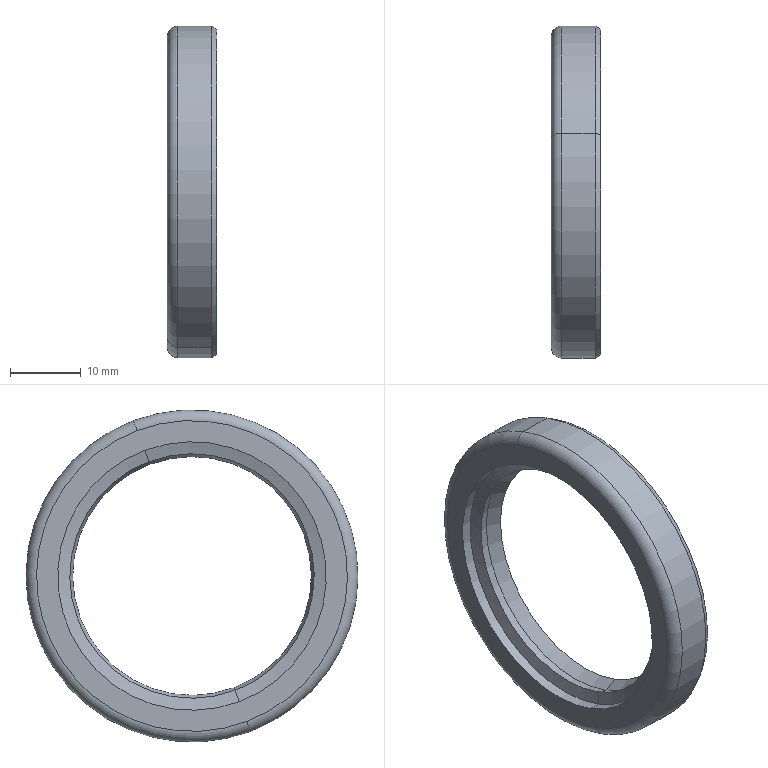Part | SolidWorks | features BaseBody 1 | 1 solid | 34 faces | box 7 x 47 x 47 mm | volume 3647 mm3 | cone 10 | cylinder 10 | torus 8 | plane 6 | commonest cylinder face diameters 38 x2 40 x2 41.6 x2 44 x2 47 x2
STEP:
#1=CARTESIAN_POINT('',(-6.4,6.861,18.253));
#2=VERTEX_POINT('',#1);
#3=CARTESIAN_POINT('',(-7.3,6.544,17.411));
#4=VERTEX_POINT('',#3);
#5=CARTESIAN_POINT('',(-7.3,6.861,18.253));
#6=DIRECTION('',(0.,0.9361,-0.3518));
#7=DIRECTION('',(0.,0.3518,0.9361));
#8=AXIS2_PLACEMENT_3D('',#5,#6,#7);
#9=CIRCLE('',#8,0.9);
#10=EDGE_CURVE('',#2,#4,#9,.T.);
#11=ORIENTED_EDGE('',*,*,#10,.T.);
#12=CARTESIAN_POINT('',(-7.3,-6.544,-17.411));
#13=VERTEX_POINT('',#12);
#14=CARTESIAN_POINT('',(-7.3,0.,0.));
#15=DIRECTION('',(1.,0.,0.));
#16=DIRECTION('',(0.,0.,-1.));
#17=AXIS2_PLACEMENT_3D('',#14,#15,#16);
#18=CIRCLE('',#17,18.6);
#19=EDGE_CURVE('',#4,#13,#18,.T.);
#20=ORIENTED_EDGE('',*,*,#19,.T.);
#21=CARTESIAN_POINT('',(-6.4,-6.861,-18.253));
#22=VERTEX_POINT('',#21);
#23=CARTESIAN_POINT('',(-7.3,-6.861,-18.253));
#24=DIRECTION('',(0.,-0.9361,0.3518));
#25=DIRECTION('',(0.,-0.3518,-0.9361));
#26=AXIS2_PLACEMENT_3D('',#23,#24,#25);
#27=CIRCLE('',#26,0.9);
#28=EDGE_CURVE('',#22,#13,#27,.T.);
#29=ORIENTED_EDGE('',*,*,#28,.F.);
#30=CARTESIAN_POINT('',(-6.4,0.,0.));
#31=DIRECTION('',(1.,0.,0.));
#32=DIRECTION('',(0.,0.3518,0.9361));
#33=AXIS2_PLACEMENT_3D('',#30,#31,#32);
#34=CIRCLE('',#33,19.5);
#35=EDGE_CURVE('',#2,#22,#34,.T.);
#36=ORIENTED_EDGE('',*,*,#35,.F.);
#37=EDGE_LOOP('',(#11,#20,#29,#36));
#38=FACE_OUTER_BOUND('',#37,.T.);
#39=CARTESIAN_POINT('',(-7.3,0.,0.));
#40=DIRECTION('',(1.,0.,0.));
#41=DIRECTION('',(0.,0.3518,0.9361));
#42=AXIS2_PLACEMENT_3D('',#39,#40,#41);
#43=TOROIDAL_SURFACE('',#42,19.5,0.9);
#44=ADVANCED_FACE('',(#38),#43,.F.);
#45=ORIENTED_EDGE('',*,*,#28,.T.);
#46=CARTESIAN_POINT('',(-7.3,0.,0.));
#47=DIRECTION('',(1.,0.,0.));
#48=DIRECTION('',(0.,0.,-1.));
#49=AXIS2_PLACEMENT_3D('',#46,#47,#48);
#50=CIRCLE('',#49,18.6);
#51=EDGE_CURVE('',#13,#4,#50,.T.);
#52=ORIENTED_EDGE('',*,*,#51,.T.);
#53=ORIENTED_EDGE('',*,*,#10,.F.);
#54=CARTESIAN_POINT('',(-6.4,0.,0.));
#55=DIRECTION('',(1.,0.,0.));
#56=DIRECTION('',(0.,0.3518,0.9361));
#57=AXIS2_PLACEMENT_3D('',#54,#55,#56);
#58=CIRCLE('',#57,19.5);
#59=EDGE_CURVE('',#22,#2,#58,.T.);
#60=ORIENTED_EDGE('',*,*,#59,.F.);
#61=EDGE_LOOP('',(#45,#52,#53,#60));
#62=FACE_OUTER_BOUND('',#61,.T.);
#63=CARTESIAN_POINT('',(-7.3,0.,0.));
#64=DIRECTION('',(1.,0.,0.));
#65=DIRECTION('',(0.,0.3518,0.9361));
#66=AXIS2_PLACEMENT_3D('',#63,#64,#65);
#67=TOROIDAL_SURFACE('',#66,19.5,0.9);
#68=ADVANCED_FACE('',(#62),#67,.F.);
#69=CARTESIAN_POINT('',(-12.,-7.741,-20.593));
#70=VERTEX_POINT('',#69);
#71=CARTESIAN_POINT('',(-12.,7.741,20.593));
#72=VERTEX_POINT('',#71);
#73=CARTESIAN_POINT('',(-12.,0.,0.));
#74=DIRECTION('',(-1.,0.,0.));
#75=DIRECTION('',(0.,0.3518,0.9361));
#76=AXIS2_PLACEMENT_3D('',#73,#74,#75);
#77=CIRCLE('',#76,22.);
#78=EDGE_CURVE('',#70,#72,#77,.T.);
#79=ORIENTED_EDGE('',*,*,#78,.F.);
#80=CARTESIAN_POINT('',(-10.5,-8.268,-21.997));
#81=VERTEX_POINT('',#80);
#82=CARTESIAN_POINT('',(-10.5,-7.741,-20.593));
#83=DIRECTION('',(0.,-0.9361,0.3518));
#84=DIRECTION('',(0.,-0.3518,-0.9361));
#85=AXIS2_PLACEMENT_3D('',#82,#83,#84);
#86=CIRCLE('',#85,1.5);
#87=EDGE_CURVE('',#70,#81,#86,.T.);
#88=ORIENTED_EDGE('',*,*,#87,.T.);
#89=CARTESIAN_POINT('',(-10.5,8.268,21.997));
#90=VERTEX_POINT('',#89);
#91=CARTESIAN_POINT('',(-10.5,0.,0.));
#92=DIRECTION('',(1.,0.,0.));
#93=DIRECTION('',(0.,0.3518,0.9361));
#94=AXIS2_PLACEMENT_3D('',#91,#92,#93);
#95=CIRCLE('',#94,23.5);
#96=EDGE_CURVE('',#90,#81,#95,.T.);
#97=ORIENTED_EDGE('',*,*,#96,.F.);
#98=CARTESIAN_POINT('',(-10.5,7.741,20.593));
#99=DIRECTION('',(0.,0.9361,-0.3518));
#100=DIRECTION('',(0.,0.3518,0.9361));
#101=AXIS2_PLACEMENT_3D('',#98,#99,#100);
#102=CIRCLE('',#101,1.5);
#103=EDGE_CURVE('',#72,#90,#102,.T.);
#104=ORIENTED_EDGE('',*,*,#103,.F.);
#105=EDGE_LOOP('',(#79,#88,#97,#104));
#106=FACE_OUTER_BOUND('',#105,.T.);
#107=CARTESIAN_POINT('',(-10.5,0.,0.));
#108=DIRECTION('',(1.,0.,0.));
#109=DIRECTION('',(0.,0.3518,0.9361));
#110=AXIS2_PLACEMENT_3D('',#107,#108,#109);
#111=TOROIDAL_SURFACE('',#110,22.,1.5);
#112=ADVANCED_FACE('',(#106),#111,.T.);
#113=CARTESIAN_POINT('',(-8.7,7.741,20.593));
#114=VERTEX_POINT('',#113);
#115=CARTESIAN_POINT('',(-8.7,-7.741,-20.593));
#116=VERTEX_POINT('',#115);
#117=CARTESIAN_POINT('',(-8.7,0.,0.));
#118=DIRECTION('',(-1.,0.,0.));
#119=DIRECTION('',(0.,-0.3518,-0.9361));
#120=AXIS2_PLACEMENT_3D('',#117,#118,#119);
#121=CIRCLE('',#120,22.);
#122=EDGE_CURVE('',#114,#116,#121,.T.);
#123=ORIENTED_EDGE('',*,*,#122,.F.);
#124=CARTESIAN_POINT('',(-9.,7.635,20.312));
#125=VERTEX_POINT('',#124);
#126=CARTESIAN_POINT('',(-8.7,7.635,20.312));
#127=DIRECTION('',(0.,-0.9361,0.3518));
#128=DIRECTION('',(0.,-0.3518,-0.9361));
#129=AXIS2_PLACEMENT_3D('',#126,#127,#128);
#130=CIRCLE('',#129,0.3);
#131=EDGE_CURVE('',#114,#125,#130,.T.);
#132=ORIENTED_EDGE('',*,*,#131,.T.);
#133=CARTESIAN_POINT('',(-9.,-7.635,-20.312));
#134=VERTEX_POINT('',#133);
#135=CARTESIAN_POINT('',(-9.,0.,0.));
#136=DIRECTION('',(1.,0.,0.));
#137=DIRECTION('',(0.,-0.3518,-0.9361));
#138=AXIS2_PLACEMENT_3D('',#135,#136,#137);
#139=CIRCLE('',#138,21.7);
#140=EDGE_CURVE('',#134,#125,#139,.T.);
#141=ORIENTED_EDGE('',*,*,#140,.F.);
#142=CARTESIAN_POINT('',(-8.7,-7.635,-20.312));
#143=DIRECTION('',(0.,0.9361,-0.3518));
#144=DIRECTION('',(0.,0.3518,0.9361));
#145=AXIS2_PLACEMENT_3D('',#142,#143,#144);
#146=CIRCLE('',#145,0.3);
#147=EDGE_CURVE('',#116,#134,#146,.T.);
#148=ORIENTED_EDGE('',*,*,#147,.F.);
#149=EDGE_LOOP('',(#123,#132,#141,#148));
#150=FACE_OUTER_BOUND('',#149,.T.);
#151=CARTESIAN_POINT('',(-8.7,0.,0.));
#152=DIRECTION('',(-1.,0.,0.));
#153=DIRECTION('',(0.,-0.3518,-0.9361));
#154=AXIS2_PLACEMENT_3D('',#151,#152,#153);
#155=TOROIDAL_SURFACE('',#154,21.7,0.3);
#156=ADVANCED_FACE('',(#150),#155,.F.);
#157=CARTESIAN_POINT('',(-5.,8.106,21.565));
#158=VERTEX_POINT('',#157);
#159=CARTESIAN_POINT('',(-5.,-8.106,-21.565));
#160=VERTEX_POINT('',#159);
#161=CARTESIAN_POINT('',(-5.,0.,0.));
#162=DIRECTION('',(1.,0.,0.));
#163=DIRECTION('',(0.,-0.3518,-0.9361));
#164=AXIS2_PLACEMENT_3D('',#161,#162,#163);
#165=CIRCLE('',#164,23.038);
#166=EDGE_CURVE('',#158,#160,#165,.T.);
#167=ORIENTED_EDGE('',*,*,#166,.F.);
#168=CARTESIAN_POINT('',(-5.8,8.268,21.997));
#169=VERTEX_POINT('',#168);
#170=CARTESIAN_POINT('',(-5.,8.106,21.565));
#171=DIRECTION('',(-0.866,0.1759,0.468));
#172=VECTOR('',#171,1000.);
#173=LINE('',#170,#172);
#174=EDGE_CURVE('',#158,#169,#173,.T.);
#175=ORIENTED_EDGE('',*,*,#174,.T.);
#176=CARTESIAN_POINT('',(-5.8,-8.268,-21.997));
#177=VERTEX_POINT('',#176);
#178=CARTESIAN_POINT('',(-5.8,0.,0.));
#179=DIRECTION('',(-1.,0.,0.));
#180=DIRECTION('',(0.,-0.3518,-0.9361));
#181=AXIS2_PLACEMENT_3D('',#178,#179,#180);
#182=CIRCLE('',#181,23.5);
#183=EDGE_CURVE('',#177,#169,#182,.T.);
#184=ORIENTED_EDGE('',*,*,#183,.F.);
#185=CARTESIAN_POINT('',(-5.,-8.106,-21.565));
#186=DIRECTION('',(-0.866,-0.1759,-0.468));
#187=VECTOR('',#186,1000.);
#188=LINE('',#185,#187);
#189=EDGE_CURVE('',#160,#177,#188,.T.);
#190=ORIENTED_EDGE('',*,*,#189,.F.);
#191=EDGE_LOOP('',(#167,#175,#184,#190));
#192=FACE_OUTER_BOUND('',#191,.T.);
#193=CARTESIAN_POINT('',(-5.,0.,0.));
#194=DIRECTION('',(-1.,0.,0.));
#195=DIRECTION('',(0.,-0.3518,-0.9361));
#196=AXIS2_PLACEMENT_3D('',#193,#194,#195);
#197=CONICAL_SURFACE('',#196,23.038,0.5236);
#198=ADVANCED_FACE('',(#192),#197,.T.);
#199=CARTESIAN_POINT('',(-9.,7.318,19.47));
#200=VERTEX_POINT('',#199);
#201=CARTESIAN_POINT('',(-9.,-7.318,-19.47));
#202=VERTEX_POINT('',#201);
#203=CARTESIAN_POINT('',(-9.,0.,0.));
#204=DIRECTION('',(1.,0.,0.));
#205=DIRECTION('',(0.,0.3518,0.9361));
#206=AXIS2_PLACEMENT_3D('',#203,#204,#205);
#207=CIRCLE('',#206,20.8);
#208=EDGE_CURVE('',#200,#202,#207,.T.);
#209=ORIENTED_EDGE('',*,*,#208,.T.);
#210=CARTESIAN_POINT('',(-8.2,-7.318,-19.47));
#211=VERTEX_POINT('',#210);
#212=CARTESIAN_POINT('',(5.743,-7.318,-19.47));
#213=DIRECTION('',(1.,0.,0.));
#214=VECTOR('',#213,1000.);
#215=LINE('',#212,#214);
#216=EDGE_CURVE('',#202,#211,#215,.T.);
#217=ORIENTED_EDGE('',*,*,#216,.T.);
#218=CARTESIAN_POINT('',(-8.2,7.318,19.47));
#219=VERTEX_POINT('',#218);
#220=CARTESIAN_POINT('',(-8.2,0.,0.));
#221=DIRECTION('',(1.,0.,0.));
#222=DIRECTION('',(0.,0.3518,0.9361));
#223=AXIS2_PLACEMENT_3D('',#220,#221,#222);
#224=CIRCLE('',#223,20.8);
#225=EDGE_CURVE('',#219,#211,#224,.T.);
#226=ORIENTED_EDGE('',*,*,#225,.F.);
#227=CARTESIAN_POINT('',(5.743,7.318,19.47));
#228=DIRECTION('',(1.,0.,0.));
#229=VECTOR('',#228,1000.);
#230=LINE('',#227,#229);
#231=EDGE_CURVE('',#200,#219,#230,.T.);
#232=ORIENTED_EDGE('',*,*,#231,.F.);
#233=EDGE_LOOP('',(#209,#217,#226,#232));
#234=FACE_OUTER_BOUND('',#233,.T.);
#235=CARTESIAN_POINT('',(5.743,0.,0.));
#236=DIRECTION('',(1.,0.,0.));
#237=DIRECTION('',(0.,0.3518,0.9361));
#238=AXIS2_PLACEMENT_3D('',#235,#236,#237);
#239=CYLINDRICAL_SURFACE('',#238,20.8);
#240=ADVANCED_FACE('',(#234),#239,.T.);
#241=ORIENTED_EDGE('',*,*,#122,.T.);
#242=CARTESIAN_POINT('',(-5.,-7.741,-20.593));
#243=VERTEX_POINT('',#242);
#244=CARTESIAN_POINT('',(5.743,-7.741,-20.593));
#245=DIRECTION('',(1.,0.,0.));
#246=VECTOR('',#245,1000.);
#247=LINE('',#244,#246);
#248=EDGE_CURVE('',#116,#243,#247,.T.);
#249=ORIENTED_EDGE('',*,*,#248,.T.);
#250=CARTESIAN_POINT('',(-5.,7.741,20.593));
#251=VERTEX_POINT('',#250);
#252=CARTESIAN_POINT('',(-5.,0.,0.));
#253=DIRECTION('',(1.,0.,0.));
#254=DIRECTION('',(0.,0.3518,0.9361));
#255=AXIS2_PLACEMENT_3D('',#252,#253,#254);
#256=CIRCLE('',#255,22.);
#257=EDGE_CURVE('',#243,#251,#256,.T.);
#258=ORIENTED_EDGE('',*,*,#257,.T.);
#259=CARTESIAN_POINT('',(5.743,7.741,20.593));
#260=DIRECTION('',(1.,0.,0.));
#261=VECTOR('',#260,1000.);
#262=LINE('',#259,#261);
#263=EDGE_CURVE('',#114,#251,#262,.T.);
#264=ORIENTED_EDGE('',*,*,#263,.F.);
#265=EDGE_LOOP('',(#241,#249,#258,#264));
#266=FACE_OUTER_BOUND('',#265,.T.);
#267=CARTESIAN_POINT('',(5.743,0.,0.));
#268=DIRECTION('',(1.,0.,0.));
#269=DIRECTION('',(0.,0.3518,0.9361));
#270=AXIS2_PLACEMENT_3D('',#267,#268,#269);
#271=CYLINDRICAL_SURFACE('',#270,22.);
#272=ADVANCED_FACE('',(#266),#271,.F.);
#273=ORIENTED_EDGE('',*,*,#96,.T.);
#274=CARTESIAN_POINT('',(5.743,-8.268,-21.997));
#275=DIRECTION('',(1.,0.,0.));
#276=VECTOR('',#275,1000.);
#277=LINE('',#274,#276);
#278=EDGE_CURVE('',#81,#177,#277,.T.);
#279=ORIENTED_EDGE('',*,*,#278,.T.);
#280=ORIENTED_EDGE('',*,*,#183,.T.);
#281=CARTESIAN_POINT('',(5.743,8.268,21.997));
#282=DIRECTION('',(1.,0.,0.));
#283=VECTOR('',#282,1000.);
#284=LINE('',#281,#283);
#285=EDGE_CURVE('',#90,#169,#284,.T.);
#286=ORIENTED_EDGE('',*,*,#285,.F.);
#287=EDGE_LOOP('',(#273,#279,#280,#286));
#288=FACE_OUTER_BOUND('',#287,.T.);
#289=CARTESIAN_POINT('',(5.743,0.,0.));
#290=DIRECTION('',(1.,0.,0.));
#291=DIRECTION('',(0.,0.3518,0.9361));
#292=AXIS2_PLACEMENT_3D('',#289,#290,#291);
#293=CYLINDRICAL_SURFACE('',#292,23.5);
#294=ADVANCED_FACE('',(#288),#293,.T.);
#295=CARTESIAN_POINT('',(-12.,-6.685,-17.785));
#296=VERTEX_POINT('',#295);
#297=CARTESIAN_POINT('',(-12.,6.685,17.785));
#298=VERTEX_POINT('',#297);
#299=CARTESIAN_POINT('',(-12.,0.,0.));
#300=DIRECTION('',(1.,0.,0.));
#301=DIRECTION('',(0.,0.3518,0.9361));
#302=AXIS2_PLACEMENT_3D('',#299,#300,#301);
#303=CIRCLE('',#302,19.);
#304=EDGE_CURVE('',#296,#298,#303,.T.);
#305=ORIENTED_EDGE('',*,*,#304,.F.);
#306=CARTESIAN_POINT('',(-10.5,-6.685,-17.785));
#307=VERTEX_POINT('',#306);
#308=CARTESIAN_POINT('',(5.743,-6.685,-17.785));
#309=DIRECTION('',(1.,0.,0.));
#310=VECTOR('',#309,1000.);
#311=LINE('',#308,#310);
#312=EDGE_CURVE('',#296,#307,#311,.T.);
#313=ORIENTED_EDGE('',*,*,#312,.T.);
#314=CARTESIAN_POINT('',(-10.5,6.685,17.785));
#315=VERTEX_POINT('',#314);
#316=CARTESIAN_POINT('',(-10.5,0.,0.));
#317=DIRECTION('',(1.,0.,0.));
#318=DIRECTION('',(0.,0.3518,0.9361));
#319=AXIS2_PLACEMENT_3D('',#316,#317,#318);
#320=CIRCLE('',#319,19.);
#321=EDGE_CURVE('',#307,#315,#320,.T.);
#322=ORIENTED_EDGE('',*,*,#321,.T.);
#323=CARTESIAN_POINT('',(5.743,6.685,17.785));
#324=DIRECTION('',(1.,0.,0.));
#325=VECTOR('',#324,1000.);
#326=LINE('',#323,#325);
#327=EDGE_CURVE('',#298,#315,#326,.T.);
#328=ORIENTED_EDGE('',*,*,#327,.F.);
#329=EDGE_LOOP('',(#305,#313,#322,#328));
#330=FACE_OUTER_BOUND('',#329,.T.);
#331=CARTESIAN_POINT('',(5.743,0.,0.));
#332=DIRECTION('',(1.,0.,0.));
#333=DIRECTION('',(0.,0.3518,0.9361));
#334=AXIS2_PLACEMENT_3D('',#331,#332,#333);
#335=CYLINDRICAL_SURFACE('',#334,19.);
#336=ADVANCED_FACE('',(#330),#335,.F.);
#337=CARTESIAN_POINT('',(-10.,-6.087,-16.194));
#338=VERTEX_POINT('',#337);
#339=CARTESIAN_POINT('',(-10.,6.087,16.194));
#340=VERTEX_POINT('',#339);
#341=CARTESIAN_POINT('',(-10.,0.,0.));
#342=DIRECTION('',(1.,0.,0.));
#343=DIRECTION('',(0.,0.3518,0.9361));
#344=AXIS2_PLACEMENT_3D('',#341,#342,#343);
#345=CIRCLE('',#344,17.3);
#346=EDGE_CURVE('',#338,#340,#345,.T.);
#347=ORIENTED_EDGE('',*,*,#346,.T.);
#348=CARTESIAN_POINT('',(-10.,6.087,16.194));
#349=DIRECTION('',(-0.2822,0.3376,0.898));
#350=VECTOR('',#349,1000.);
#351=LINE('',#348,#350);
#352=EDGE_CURVE('',#340,#315,#351,.T.);
#353=ORIENTED_EDGE('',*,*,#352,.T.);
#354=ORIENTED_EDGE('',*,*,#321,.F.);
#355=CARTESIAN_POINT('',(-10.,-6.087,-16.194));
#356=DIRECTION('',(-0.2822,-0.3376,-0.898));
#357=VECTOR('',#356,1000.);
#358=LINE('',#355,#357);
#359=EDGE_CURVE('',#338,#307,#358,.T.);
#360=ORIENTED_EDGE('',*,*,#359,.F.);
#361=EDGE_LOOP('',(#347,#353,#354,#360));
#362=FACE_OUTER_BOUND('',#361,.T.);
#363=CARTESIAN_POINT('',(-10.,0.,0.));
#364=DIRECTION('',(-1.,0.,0.));
#365=DIRECTION('',(0.,-0.3518,-0.9361));
#366=AXIS2_PLACEMENT_3D('',#363,#364,#365);
#367=CONICAL_SURFACE('',#366,17.3,1.285);
#368=ADVANCED_FACE('',(#362),#367,.F.);
#369=ORIENTED_EDGE('',*,*,#346,.F.);
#370=CARTESIAN_POINT('',(-8.5,-6.242,-16.607));
#371=VERTEX_POINT('',#370);
#372=CARTESIAN_POINT('',(-8.5,-6.242,-16.607));
#373=DIRECTION('',(0.9594,-0.09928,-0.2641));
#374=VECTOR('',#373,1000.);
#375=LINE('',#372,#374);
#376=EDGE_CURVE('',#338,#371,#375,.T.);
#377=ORIENTED_EDGE('',*,*,#376,.T.);
#378=CARTESIAN_POINT('',(-8.5,6.242,16.607));
#379=VERTEX_POINT('',#378);
#380=CARTESIAN_POINT('',(-8.5,0.,0.));
#381=DIRECTION('',(1.,0.,0.));
#382=DIRECTION('',(0.,0.3518,0.9361));
#383=AXIS2_PLACEMENT_3D('',#380,#381,#382);
#384=CIRCLE('',#383,17.741);
#385=EDGE_CURVE('',#371,#379,#384,.T.);
#386=ORIENTED_EDGE('',*,*,#385,.T.);
#387=CARTESIAN_POINT('',(-8.5,6.242,16.607));
#388=DIRECTION('',(0.9594,0.09928,0.2641));
#389=VECTOR('',#388,1000.);
#390=LINE('',#387,#389);
#391=EDGE_CURVE('',#340,#379,#390,.T.);
#392=ORIENTED_EDGE('',*,*,#391,.F.);
#393=EDGE_LOOP('',(#369,#377,#386,#392));
#394=FACE_OUTER_BOUND('',#393,.T.);
#395=CARTESIAN_POINT('',(-8.5,0.,0.));
#396=DIRECTION('',(1.,0.,0.));
#397=DIRECTION('',(0.,0.3518,0.9361));
#398=AXIS2_PLACEMENT_3D('',#395,#396,#397);
#399=CONICAL_SURFACE('',#398,17.741,0.2861);
#400=ADVANCED_FACE('',(#394),#399,.F.);
#401=CARTESIAN_POINT('',(-6.5,-5.946,-15.819));
#402=VERTEX_POINT('',#401);
#403=CARTESIAN_POINT('',(-6.5,5.946,15.819));
#404=VERTEX_POINT('',#403);
#405=CARTESIAN_POINT('',(-6.5,0.,0.));
#406=DIRECTION('',(1.,0.,0.));
#407=DIRECTION('',(0.,0.3518,0.9361));
#408=AXIS2_PLACEMENT_3D('',#405,#406,#407);
#409=CIRCLE('',#408,16.9);
#410=EDGE_CURVE('',#402,#404,#409,.T.);
#411=ORIENTED_EDGE('',*,*,#410,.T.);
#412=CARTESIAN_POINT('',(-6.5,5.946,15.819));
#413=DIRECTION('',(-0.9218,0.1364,0.3629));
#414=VECTOR('',#413,1000.);
#415=LINE('',#412,#414);
#416=EDGE_CURVE('',#404,#379,#415,.T.);
#417=ORIENTED_EDGE('',*,*,#416,.T.);
#418=ORIENTED_EDGE('',*,*,#385,.F.);
#419=CARTESIAN_POINT('',(-6.5,-5.946,-15.819));
#420=DIRECTION('',(-0.9218,-0.1364,-0.3629));
#421=VECTOR('',#420,1000.);
#422=LINE('',#419,#421);
#423=EDGE_CURVE('',#402,#371,#422,.T.);
#424=ORIENTED_EDGE('',*,*,#423,.F.);
#425=EDGE_LOOP('',(#411,#417,#418,#424));
#426=FACE_OUTER_BOUND('',#425,.T.);
#427=CARTESIAN_POINT('',(-6.5,0.,0.));
#428=DIRECTION('',(-1.,0.,0.));
#429=DIRECTION('',(0.,-0.3518,-0.9361));
#430=AXIS2_PLACEMENT_3D('',#427,#428,#429);
#431=CONICAL_SURFACE('',#430,16.9,0.3981);
#432=ADVANCED_FACE('',(#426),#431,.F.);
#433=ORIENTED_EDGE('',*,*,#410,.F.);
#434=CARTESIAN_POINT('',(-5.5,-6.515,-17.332));
#435=VERTEX_POINT('',#434);
#436=CARTESIAN_POINT('',(-5.5,-6.515,-17.332));
#437=DIRECTION('',(0.5261,-0.2992,-0.796));
#438=VECTOR('',#437,1000.);
#439=LINE('',#436,#438);
#440=EDGE_CURVE('',#402,#435,#439,.T.);
#441=ORIENTED_EDGE('',*,*,#440,.T.);
#442=CARTESIAN_POINT('',(-5.5,6.515,17.332));
#443=VERTEX_POINT('',#442);
#444=CARTESIAN_POINT('',(-5.5,0.,0.));
#445=DIRECTION('',(1.,0.,0.));
#446=DIRECTION('',(0.,0.3518,0.9361));
#447=AXIS2_PLACEMENT_3D('',#444,#445,#446);
#448=CIRCLE('',#447,18.516);
#449=EDGE_CURVE('',#435,#443,#448,.T.);
#450=ORIENTED_EDGE('',*,*,#449,.T.);
#451=CARTESIAN_POINT('',(-5.5,6.515,17.332));
#452=DIRECTION('',(0.5261,0.2992,0.796));
#453=VECTOR('',#452,1000.);
#454=LINE('',#451,#453);
#455=EDGE_CURVE('',#404,#443,#454,.T.);
#456=ORIENTED_EDGE('',*,*,#455,.F.);
#457=EDGE_LOOP('',(#433,#441,#450,#456));
#458=FACE_OUTER_BOUND('',#457,.T.);
#459=CARTESIAN_POINT('',(-5.5,0.,0.));
#460=DIRECTION('',(1.,0.,0.));
#461=DIRECTION('',(0.,0.3518,0.9361));
#462=AXIS2_PLACEMENT_3D('',#459,#460,#461);
#463=CONICAL_SURFACE('',#462,18.516,1.017);
#464=ADVANCED_FACE('',(#458),#463,.F.);
#465=CARTESIAN_POINT('',(-6.4,7.037,18.721));
#466=VERTEX_POINT('',#465);
#467=CARTESIAN_POINT('',(-6.4,-7.037,-18.721));
#468=VERTEX_POINT('',#467);
#469=CARTESIAN_POINT('',(-6.4,0.,0.));
#470=DIRECTION('',(1.,0.,0.));
#471=DIRECTION('',(0.,0.3518,0.9361));
#472=AXIS2_PLACEMENT_3D('',#469,#470,#471);
#473=CIRCLE('',#472,20.);
#474=EDGE_CURVE('',#466,#468,#473,.T.);
#475=ORIENTED_EDGE('',*,*,#474,.T.);
#476=CARTESIAN_POINT('',(-5.5,-7.037,-18.721));
#477=VERTEX_POINT('',#476);
#478=CARTESIAN_POINT('',(5.743,-7.037,-18.721));
#479=DIRECTION('',(1.,0.,0.));
#480=VECTOR('',#479,1000.);
#481=LINE('',#478,#480);
#482=EDGE_CURVE('',#468,#477,#481,.T.);
#483=ORIENTED_EDGE('',*,*,#482,.T.);
#484=CARTESIAN_POINT('',(-5.5,7.037,18.721));
#485=VERTEX_POINT('',#484);
#486=CARTESIAN_POINT('',(-5.5,0.,0.));
#487=DIRECTION('',(1.,0.,0.));
#488=DIRECTION('',(0.,0.3518,0.9361));
#489=AXIS2_PLACEMENT_3D('',#486,#487,#488);
#490=CIRCLE('',#489,20.);
#491=EDGE_CURVE('',#485,#477,#490,.T.);
#492=ORIENTED_EDGE('',*,*,#491,.F.);
#493=CARTESIAN_POINT('',(5.743,7.037,18.721));
#494=DIRECTION('',(1.,0.,0.));
#495=VECTOR('',#494,1000.);
#496=LINE('',#493,#495);
#497=EDGE_CURVE('',#466,#485,#496,.T.);
#498=ORIENTED_EDGE('',*,*,#497,.F.);
#499=EDGE_LOOP('',(#475,#483,#492,#498));
#500=FACE_OUTER_BOUND('',#499,.T.);
#501=CARTESIAN_POINT('',(5.743,0.,0.));
#502=DIRECTION('',(1.,0.,0.));
#503=DIRECTION('',(0.,0.3518,0.9361));
#504=AXIS2_PLACEMENT_3D('',#501,#502,#503);
#505=CYLINDRICAL_SURFACE('',#504,20.);
#506=ADVANCED_FACE('',(#500),#505,.T.);
#507=ORIENTED_EDGE('',*,*,#51,.F.);
#508=CARTESIAN_POINT('',(-8.2,-6.861,-18.253));
#509=VERTEX_POINT('',#508);
#510=CARTESIAN_POINT('',(-7.3,-6.861,-18.253));
#511=DIRECTION('',(0.,-0.9361,0.3518));
#512=DIRECTION('',(0.,-0.3518,-0.9361));
#513=AXIS2_PLACEMENT_3D('',#510,#511,#512);
#514=CIRCLE('',#513,0.9);
#515=EDGE_CURVE('',#13,#509,#514,.T.);
#516=ORIENTED_EDGE('',*,*,#515,.T.);
#517=CARTESIAN_POINT('',(-8.2,6.861,18.253));
#518=VERTEX_POINT('',#517);
#519=CARTESIAN_POINT('',(-8.2,0.,0.));
#520=DIRECTION('',(1.,0.,0.));
#521=DIRECTION('',(0.,0.3518,0.9361));
#522=AXIS2_PLACEMENT_3D('',#519,#520,#521);
#523=CIRCLE('',#522,19.5);
#524=EDGE_CURVE('',#509,#518,#523,.T.);
#525=ORIENTED_EDGE('',*,*,#524,.T.);
#526=CARTESIAN_POINT('',(-7.3,6.861,18.253));
#527=DIRECTION('',(0.,0.9361,-0.3518));
#528=DIRECTION('',(0.,0.3518,0.9361));
#529=AXIS2_PLACEMENT_3D('',#526,#527,#528);
#530=CIRCLE('',#529,0.9);
#531=EDGE_CURVE('',#4,#518,#530,.T.);
#532=ORIENTED_EDGE('',*,*,#531,.F.);
#533=EDGE_LOOP('',(#507,#516,#525,#532));
#534=FACE_OUTER_BOUND('',#533,.T.);
#535=CARTESIAN_POINT('',(-7.3,0.,0.));
#536=DIRECTION('',(1.,0.,0.));
#537=DIRECTION('',(0.,0.3518,0.9361));
#538=AXIS2_PLACEMENT_3D('',#535,#536,#537);
#539=TOROIDAL_SURFACE('',#538,19.5,0.9);
#540=ADVANCED_FACE('',(#534),#539,.F.);
#541=ORIENTED_EDGE('',*,*,#19,.F.);
#542=ORIENTED_EDGE('',*,*,#531,.T.);
#543=CARTESIAN_POINT('',(-8.2,0.,0.));
#544=DIRECTION('',(1.,0.,0.));
#545=DIRECTION('',(0.,0.3518,0.9361));
#546=AXIS2_PLACEMENT_3D('',#543,#544,#545);
#547=CIRCLE('',#546,19.5);
#548=EDGE_CURVE('',#518,#509,#547,.T.);
#549=ORIENTED_EDGE('',*,*,#548,.T.);
#550=ORIENTED_EDGE('',*,*,#515,.F.);
#551=EDGE_LOOP('',(#541,#542,#549,#550));
#552=FACE_OUTER_BOUND('',#551,.T.);
#553=CARTESIAN_POINT('',(-7.3,0.,0.));
#554=DIRECTION('',(1.,0.,0.));
#555=DIRECTION('',(0.,0.3518,0.9361));
#556=AXIS2_PLACEMENT_3D('',#553,#554,#555);
#557=TOROIDAL_SURFACE('',#556,19.5,0.9);
#558=ADVANCED_FACE('',(#552),#557,.F.);
#559=ORIENTED_EDGE('',*,*,#35,.T.);
#560=ORIENTED_EDGE('',*,*,#59,.T.);
#561=EDGE_LOOP('',(#559,#560));
#562=FACE_BOUND('',#561,.T.);
#563=ORIENTED_EDGE('',*,*,#474,.F.);
#564=CARTESIAN_POINT('',(-6.4,0.,0.));
#565=DIRECTION('',(1.,0.,0.));
#566=DIRECTION('',(0.,0.3518,0.9361));
#567=AXIS2_PLACEMENT_3D('',#564,#565,#566);
#568=CIRCLE('',#567,20.);
#569=EDGE_CURVE('',#468,#466,#568,.T.);
#570=ORIENTED_EDGE('',*,*,#569,.F.);
#571=EDGE_LOOP('',(#563,#570));
#572=FACE_OUTER_BOUND('',#571,.T.);
#573=CARTESIAN_POINT('',(-6.4,-11.155,4.193));
#574=DIRECTION('',(-1.,0.,0.));
#575=DIRECTION('',(0.,-0.3518,-0.9361));
#576=AXIS2_PLACEMENT_3D('',#573,#574,#575);
#577=PLANE('',#576);
#578=ADVANCED_FACE('',(#562,#572),#577,.T.);
#579=ORIENTED_EDGE('',*,*,#482,.F.);
#580=ORIENTED_EDGE('',*,*,#569,.T.);
#581=ORIENTED_EDGE('',*,*,#497,.T.);
#582=CARTESIAN_POINT('',(-5.5,0.,0.));
#583=DIRECTION('',(1.,0.,0.));
#584=DIRECTION('',(0.,0.3518,0.9361));
#585=AXIS2_PLACEMENT_3D('',#582,#583,#584);
#586=CIRCLE('',#585,20.);
#587=EDGE_CURVE('',#477,#485,#586,.T.);
#588=ORIENTED_EDGE('',*,*,#587,.F.);
#589=EDGE_LOOP('',(#579,#580,#581,#588));
#590=FACE_OUTER_BOUND('',#589,.T.);
#591=CARTESIAN_POINT('',(5.743,0.,0.));
#592=DIRECTION('',(1.,0.,0.));
#593=DIRECTION('',(0.,0.3518,0.9361));
#594=AXIS2_PLACEMENT_3D('',#591,#592,#593);
#595=CYLINDRICAL_SURFACE('',#594,20.);
#596=ADVANCED_FACE('',(#590),#595,.T.);
#597=CARTESIAN_POINT('',(-5.5,0.,0.));
#598=DIRECTION('',(1.,0.,0.));
#599=DIRECTION('',(0.,0.3518,0.9361));
#600=AXIS2_PLACEMENT_3D('',#597,#598,#599);
#601=CIRCLE('',#600,18.516);
#602=EDGE_CURVE('',#443,#435,#601,.T.);
#603=ORIENTED_EDGE('',*,*,#602,.F.);
#604=ORIENTED_EDGE('',*,*,#449,.F.);
#605=EDGE_LOOP('',(#603,#604));
#606=FACE_BOUND('',#605,.T.);
#607=ORIENTED_EDGE('',*,*,#491,.T.);
#608=ORIENTED_EDGE('',*,*,#587,.T.);
#609=EDGE_LOOP('',(#607,#608));
#610=FACE_OUTER_BOUND('',#609,.T.);
#611=CARTESIAN_POINT('',(-5.5,-11.155,4.193));
#612=DIRECTION('',(-1.,0.,0.));
#613=DIRECTION('',(0.,-0.3518,-0.9361));
#614=AXIS2_PLACEMENT_3D('',#611,#612,#613);
#615=PLANE('',#614);
#616=ADVANCED_FACE('',(#606,#610),#615,.F.);
#617=ORIENTED_EDGE('',*,*,#440,.F.);
#618=CARTESIAN_POINT('',(-6.5,0.,0.));
#619=DIRECTION('',(1.,0.,0.));
#620=DIRECTION('',(0.,0.3518,0.9361));
#621=AXIS2_PLACEMENT_3D('',#618,#619,#620);
#622=CIRCLE('',#621,16.9);
#623=EDGE_CURVE('',#404,#402,#622,.T.);
#624=ORIENTED_EDGE('',*,*,#623,.F.);
#625=ORIENTED_EDGE('',*,*,#455,.T.);
#626=ORIENTED_EDGE('',*,*,#602,.T.);
#627=EDGE_LOOP('',(#617,#624,#625,#626));
#628=FACE_OUTER_BOUND('',#627,.T.);
#629=CARTESIAN_POINT('',(-5.5,0.,0.));
#630=DIRECTION('',(1.,0.,0.));
#631=DIRECTION('',(0.,0.3518,0.9361));
#632=AXIS2_PLACEMENT_3D('',#629,#630,#631);
#633=CONICAL_SURFACE('',#632,18.516,1.017);
#634=ADVANCED_FACE('',(#628),#633,.F.);
#635=ORIENTED_EDGE('',*,*,#416,.F.);
#636=ORIENTED_EDGE('',*,*,#623,.T.);
#637=ORIENTED_EDGE('',*,*,#423,.T.);
#638=CARTESIAN_POINT('',(-8.5,0.,0.));
#639=DIRECTION('',(1.,0.,0.));
#640=DIRECTION('',(0.,0.3518,0.9361));
#641=AXIS2_PLACEMENT_3D('',#638,#639,#640);
#642=CIRCLE('',#641,17.741);
#643=EDGE_CURVE('',#379,#371,#642,.T.);
#644=ORIENTED_EDGE('',*,*,#643,.F.);
#645=EDGE_LOOP('',(#635,#636,#637,#644));
#646=FACE_OUTER_BOUND('',#645,.T.);
#647=CARTESIAN_POINT('',(-6.5,0.,0.));
#648=DIRECTION('',(-1.,0.,0.));
#649=DIRECTION('',(0.,-0.3518,-0.9361));
#650=AXIS2_PLACEMENT_3D('',#647,#648,#649);
#651=CONICAL_SURFACE('',#650,16.9,0.3981);
#652=ADVANCED_FACE('',(#646),#651,.F.);
#653=ORIENTED_EDGE('',*,*,#376,.F.);
#654=CARTESIAN_POINT('',(-10.,0.,0.));
#655=DIRECTION('',(1.,0.,0.));
#656=DIRECTION('',(0.,0.3518,0.9361));
#657=AXIS2_PLACEMENT_3D('',#654,#655,#656);
#658=CIRCLE('',#657,17.3);
#659=EDGE_CURVE('',#340,#338,#658,.T.);
#660=ORIENTED_EDGE('',*,*,#659,.F.);
#661=ORIENTED_EDGE('',*,*,#391,.T.);
#662=ORIENTED_EDGE('',*,*,#643,.T.);
#663=EDGE_LOOP('',(#653,#660,#661,#662));
#664=FACE_OUTER_BOUND('',#663,.T.);
#665=CARTESIAN_POINT('',(-8.5,0.,0.));
#666=DIRECTION('',(1.,0.,0.));
#667=DIRECTION('',(0.,0.3518,0.9361));
#668=AXIS2_PLACEMENT_3D('',#665,#666,#667);
#669=CONICAL_SURFACE('',#668,17.741,0.2861);
#670=ADVANCED_FACE('',(#664),#669,.F.);
#671=ORIENTED_EDGE('',*,*,#352,.F.);
#672=ORIENTED_EDGE('',*,*,#659,.T.);
#673=ORIENTED_EDGE('',*,*,#359,.T.);
#674=CARTESIAN_POINT('',(-10.5,0.,0.));
#675=DIRECTION('',(1.,0.,0.));
#676=DIRECTION('',(0.,0.3518,0.9361));
#677=AXIS2_PLACEMENT_3D('',#674,#675,#676);
#678=CIRCLE('',#677,19.);
#679=EDGE_CURVE('',#315,#307,#678,.T.);
#680=ORIENTED_EDGE('',*,*,#679,.F.);
#681=EDGE_LOOP('',(#671,#672,#673,#680));
#682=FACE_OUTER_BOUND('',#681,.T.);
#683=CARTESIAN_POINT('',(-10.,0.,0.));
#684=DIRECTION('',(-1.,0.,0.));
#685=DIRECTION('',(0.,-0.3518,-0.9361));
#686=AXIS2_PLACEMENT_3D('',#683,#684,#685);
#687=CONICAL_SURFACE('',#686,17.3,1.285);
#688=ADVANCED_FACE('',(#682),#687,.F.);
#689=ORIENTED_EDGE('',*,*,#312,.F.);
#690=CARTESIAN_POINT('',(-12.,0.,0.));
#691=DIRECTION('',(1.,0.,0.));
#692=DIRECTION('',(0.,0.3518,0.9361));
#693=AXIS2_PLACEMENT_3D('',#690,#691,#692);
#694=CIRCLE('',#693,19.);
#695=EDGE_CURVE('',#298,#296,#694,.T.);
#696=ORIENTED_EDGE('',*,*,#695,.F.);
#697=ORIENTED_EDGE('',*,*,#327,.T.);
#698=ORIENTED_EDGE('',*,*,#679,.T.);
#699=EDGE_LOOP('',(#689,#696,#697,#698));
#700=FACE_OUTER_BOUND('',#699,.T.);
#701=CARTESIAN_POINT('',(5.743,0.,0.));
#702=DIRECTION('',(1.,0.,0.));
#703=DIRECTION('',(0.,0.3518,0.9361));
#704=AXIS2_PLACEMENT_3D('',#701,#702,#703);
#705=CYLINDRICAL_SURFACE('',#704,19.);
#706=ADVANCED_FACE('',(#700),#705,.F.);
#707=CARTESIAN_POINT('',(-12.,0.,0.));
#708=DIRECTION('',(-1.,0.,0.));
#709=DIRECTION('',(0.,0.3518,0.9361));
#710=AXIS2_PLACEMENT_3D('',#707,#708,#709);
#711=CIRCLE('',#710,22.);
#712=EDGE_CURVE('',#72,#70,#711,.T.);
#713=ORIENTED_EDGE('',*,*,#712,.T.);
#714=ORIENTED_EDGE('',*,*,#78,.T.);
#715=EDGE_LOOP('',(#713,#714));
#716=FACE_OUTER_BOUND('',#715,.T.);
#717=ORIENTED_EDGE('',*,*,#695,.T.);
#718=ORIENTED_EDGE('',*,*,#304,.T.);
#719=EDGE_LOOP('',(#717,#718));
#720=FACE_BOUND('',#719,.T.);
#721=CARTESIAN_POINT('',(-12.,-11.155,4.193));
#722=DIRECTION('',(1.,0.,0.));
#723=DIRECTION('',(0.,0.3518,0.9361));
#724=AXIS2_PLACEMENT_3D('',#721,#722,#723);
#725=PLANE('',#724);
#726=ADVANCED_FACE('',(#716,#720),#725,.F.);
#727=ORIENTED_EDGE('',*,*,#278,.F.);
#728=CARTESIAN_POINT('',(-10.5,0.,0.));
#729=DIRECTION('',(1.,0.,0.));
#730=DIRECTION('',(0.,0.3518,0.9361));
#731=AXIS2_PLACEMENT_3D('',#728,#729,#730);
#732=CIRCLE('',#731,23.5);
#733=EDGE_CURVE('',#81,#90,#732,.T.);
#734=ORIENTED_EDGE('',*,*,#733,.T.);
#735=ORIENTED_EDGE('',*,*,#285,.T.);
#736=CARTESIAN_POINT('',(-5.8,0.,0.));
#737=DIRECTION('',(-1.,0.,0.));
#738=DIRECTION('',(0.,-0.3518,-0.9361));
#739=AXIS2_PLACEMENT_3D('',#736,#737,#738);
#740=CIRCLE('',#739,23.5);
#741=EDGE_CURVE('',#169,#177,#740,.T.);
#742=ORIENTED_EDGE('',*,*,#741,.T.);
#743=EDGE_LOOP('',(#727,#734,#735,#742));
#744=FACE_OUTER_BOUND('',#743,.T.);
#745=CARTESIAN_POINT('',(5.743,0.,0.));
#746=DIRECTION('',(1.,0.,0.));
#747=DIRECTION('',(0.,0.3518,0.9361));
#748=AXIS2_PLACEMENT_3D('',#745,#746,#747);
#749=CYLINDRICAL_SURFACE('',#748,23.5);
#750=ADVANCED_FACE('',(#744),#749,.T.);
#751=CARTESIAN_POINT('',(-5.,0.,0.));
#752=DIRECTION('',(1.,0.,0.));
#753=DIRECTION('',(0.,-0.3518,-0.9361));
#754=AXIS2_PLACEMENT_3D('',#751,#752,#753);
#755=CIRCLE('',#754,23.038);
#756=EDGE_CURVE('',#160,#158,#755,.T.);
#757=ORIENTED_EDGE('',*,*,#756,.T.);
#758=ORIENTED_EDGE('',*,*,#166,.T.);
#759=EDGE_LOOP('',(#757,#758));
#760=FACE_OUTER_BOUND('',#759,.T.);
#761=CARTESIAN_POINT('',(-5.,0.,0.));
#762=DIRECTION('',(1.,0.,0.));
#763=DIRECTION('',(0.,0.3518,0.9361));
#764=AXIS2_PLACEMENT_3D('',#761,#762,#763);
#765=CIRCLE('',#764,22.);
#766=EDGE_CURVE('',#251,#243,#765,.T.);
#767=ORIENTED_EDGE('',*,*,#766,.F.);
#768=ORIENTED_EDGE('',*,*,#257,.F.);
#769=EDGE_LOOP('',(#767,#768));
#770=FACE_BOUND('',#769,.T.);
#771=CARTESIAN_POINT('',(-5.,-11.155,4.193));
#772=DIRECTION('',(-1.,0.,0.));
#773=DIRECTION('',(0.,-0.3518,-0.9361));
#774=AXIS2_PLACEMENT_3D('',#771,#772,#773);
#775=PLANE('',#774);
#776=ADVANCED_FACE('',(#760,#770),#775,.F.);
#777=ORIENTED_EDGE('',*,*,#248,.F.);
#778=CARTESIAN_POINT('',(-8.7,0.,0.));
#779=DIRECTION('',(-1.,0.,0.));
#780=DIRECTION('',(0.,-0.3518,-0.9361));
#781=AXIS2_PLACEMENT_3D('',#778,#779,#780);
#782=CIRCLE('',#781,22.);
#783=EDGE_CURVE('',#116,#114,#782,.T.);
#784=ORIENTED_EDGE('',*,*,#783,.T.);
#785=ORIENTED_EDGE('',*,*,#263,.T.);
#786=ORIENTED_EDGE('',*,*,#766,.T.);
#787=EDGE_LOOP('',(#777,#784,#785,#786));
#788=FACE_OUTER_BOUND('',#787,.T.);
#789=CARTESIAN_POINT('',(5.743,0.,0.));
#790=DIRECTION('',(1.,0.,0.));
#791=DIRECTION('',(0.,0.3518,0.9361));
#792=AXIS2_PLACEMENT_3D('',#789,#790,#791);
#793=CYLINDRICAL_SURFACE('',#792,22.);
#794=ADVANCED_FACE('',(#788),#793,.F.);
#795=ORIENTED_EDGE('',*,*,#140,.T.);
#796=CARTESIAN_POINT('',(-9.,0.,0.));
#797=DIRECTION('',(1.,0.,0.));
#798=DIRECTION('',(0.,-0.3518,-0.9361));
#799=AXIS2_PLACEMENT_3D('',#796,#797,#798);
#800=CIRCLE('',#799,21.7);
#801=EDGE_CURVE('',#125,#134,#800,.T.);
#802=ORIENTED_EDGE('',*,*,#801,.T.);
#803=EDGE_LOOP('',(#795,#802));
#804=FACE_OUTER_BOUND('',#803,.T.);
#805=ORIENTED_EDGE('',*,*,#208,.F.);
#806=CARTESIAN_POINT('',(-9.,0.,0.));
#807=DIRECTION('',(1.,0.,0.));
#808=DIRECTION('',(0.,0.3518,0.9361));
#809=AXIS2_PLACEMENT_3D('',#806,#807,#808);
#810=CIRCLE('',#809,20.8);
#811=EDGE_CURVE('',#202,#200,#810,.T.);
#812=ORIENTED_EDGE('',*,*,#811,.F.);
#813=EDGE_LOOP('',(#805,#812));
#814=FACE_BOUND('',#813,.T.);
#815=CARTESIAN_POINT('',(-9.,-11.155,4.193));
#816=DIRECTION('',(-1.,0.,0.));
#817=DIRECTION('',(0.,-0.3518,-0.9361));
#818=AXIS2_PLACEMENT_3D('',#815,#816,#817);
#819=PLANE('',#818);
#820=ADVANCED_FACE('',(#804,#814),#819,.F.);
#821=ORIENTED_EDGE('',*,*,#216,.F.);
#822=ORIENTED_EDGE('',*,*,#811,.T.);
#823=ORIENTED_EDGE('',*,*,#231,.T.);
#824=CARTESIAN_POINT('',(-8.2,0.,0.));
#825=DIRECTION('',(1.,0.,0.));
#826=DIRECTION('',(0.,0.3518,0.9361));
#827=AXIS2_PLACEMENT_3D('',#824,#825,#826);
#828=CIRCLE('',#827,20.8);
#829=EDGE_CURVE('',#211,#219,#828,.T.);
#830=ORIENTED_EDGE('',*,*,#829,.F.);
#831=EDGE_LOOP('',(#821,#822,#823,#830));
#832=FACE_OUTER_BOUND('',#831,.T.);
#833=CARTESIAN_POINT('',(5.743,0.,0.));
#834=DIRECTION('',(1.,0.,0.));
#835=DIRECTION('',(0.,0.3518,0.9361));
#836=AXIS2_PLACEMENT_3D('',#833,#834,#835);
#837=CYLINDRICAL_SURFACE('',#836,20.8);
#838=ADVANCED_FACE('',(#832),#837,.T.);
#839=ORIENTED_EDGE('',*,*,#548,.F.);
#840=ORIENTED_EDGE('',*,*,#524,.F.);
#841=EDGE_LOOP('',(#839,#840));
#842=FACE_BOUND('',#841,.T.);
#843=ORIENTED_EDGE('',*,*,#225,.T.);
#844=ORIENTED_EDGE('',*,*,#829,.T.);
#845=EDGE_LOOP('',(#843,#844));
#846=FACE_OUTER_BOUND('',#845,.T.);
#847=CARTESIAN_POINT('',(-8.2,-11.155,4.193));
#848=DIRECTION('',(-1.,0.,0.));
#849=DIRECTION('',(0.,-0.3518,-0.9361));
#850=AXIS2_PLACEMENT_3D('',#847,#848,#849);
#851=PLANE('',#850);
#852=ADVANCED_FACE('',(#842,#846),#851,.F.);
#853=ORIENTED_EDGE('',*,*,#174,.F.);
#854=ORIENTED_EDGE('',*,*,#756,.F.);
#855=ORIENTED_EDGE('',*,*,#189,.T.);
#856=ORIENTED_EDGE('',*,*,#741,.F.);
#857=EDGE_LOOP('',(#853,#854,#855,#856));
#858=FACE_OUTER_BOUND('',#857,.T.);
#859=CARTESIAN_POINT('',(-5.,0.,0.));
#860=DIRECTION('',(-1.,0.,0.));
#861=DIRECTION('',(0.,-0.3518,-0.9361));
#862=AXIS2_PLACEMENT_3D('',#859,#860,#861);
#863=CONICAL_SURFACE('',#862,23.038,0.5236);
#864=ADVANCED_FACE('',(#858),#863,.T.);
#865=ORIENTED_EDGE('',*,*,#131,.F.);
#866=ORIENTED_EDGE('',*,*,#783,.F.);
#867=ORIENTED_EDGE('',*,*,#147,.T.);
#868=ORIENTED_EDGE('',*,*,#801,.F.);
#869=EDGE_LOOP('',(#865,#866,#867,#868));
#870=FACE_OUTER_BOUND('',#869,.T.);
#871=CARTESIAN_POINT('',(-8.7,0.,0.));
#872=DIRECTION('',(-1.,0.,0.));
#873=DIRECTION('',(0.,-0.3518,-0.9361));
#874=AXIS2_PLACEMENT_3D('',#871,#872,#873);
#875=TOROIDAL_SURFACE('',#874,21.7,0.3);
#876=ADVANCED_FACE('',(#870),#875,.F.);
#877=ORIENTED_EDGE('',*,*,#87,.F.);
#878=ORIENTED_EDGE('',*,*,#712,.F.);
#879=ORIENTED_EDGE('',*,*,#103,.T.);
#880=ORIENTED_EDGE('',*,*,#733,.F.);
#881=EDGE_LOOP('',(#877,#878,#879,#880));
#882=FACE_OUTER_BOUND('',#881,.T.);
#883=CARTESIAN_POINT('',(-10.5,0.,0.));
#884=DIRECTION('',(1.,0.,0.));
#885=DIRECTION('',(0.,0.3518,0.9361));
#886=AXIS2_PLACEMENT_3D('',#883,#884,#885);
#887=TOROIDAL_SURFACE('',#886,22.,1.5);
#888=ADVANCED_FACE('',(#882),#887,.T.);
#889=CLOSED_SHELL('',(#44,#68,#112,#156,#198,#240,#272,#294,#336,#368,#400,#432,#464,#506,#540,#558,#578,#596,#616,#634,#652,#670,#688,#706,#726,#750,#776,#794,#820,#838,#852,#864,#876,#888));
#890=MANIFOLD_SOLID_BREP('',#889);
#891=CARTESIAN_POINT('',(0.,0.,0.));
#892=DIRECTION('',(0.,0.,1.));
#893=DIRECTION('',(1.,0.,0.));
#894=AXIS2_PLACEMENT_3D('',#891,#892,#893);
#895=(LENGTH_UNIT()NAMED_UNIT(*)SI_UNIT(.MILLI.,.METRE.));
#896=UNCERTAINTY_MEASURE_WITH_UNIT(LENGTH_MEASURE(0.00001),#895,'','');
#897=(NAMED_UNIT(*)PLANE_ANGLE_UNIT()SI_UNIT($,.RADIAN.));
#898=(NAMED_UNIT(*)SI_UNIT($,.STERADIAN.)SOLID_ANGLE_UNIT());
#899=(GEOMETRIC_REPRESENTATION_CONTEXT(3)GLOBAL_UNCERTAINTY_ASSIGNED_CONTEXT((#896))GLOBAL_UNIT_ASSIGNED_CONTEXT((#895,#897,#898))REPRESENTATION_CONTEXT('',''));
#900=ADVANCED_BREP_SHAPE_REPRESENTATION('',(#890,#894),#899);